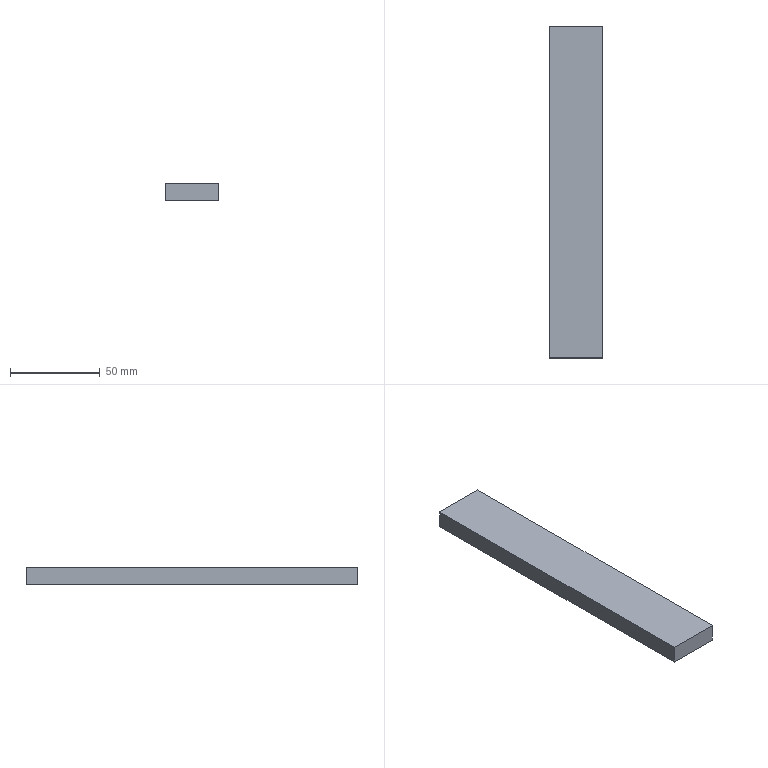Part | NX | features solid 2 | 1 solid | 6 faces | box 30 x 185 x 10 mm | volume 55500 mm3 | plane 6
STEP:
#1=CARTESIAN_POINT('',(665.,-225.,10.));
#2=VERTEX_POINT('',#1);
#3=CARTESIAN_POINT('',(665.,-225.,20.));
#4=VERTEX_POINT('',#3);
#5=CARTESIAN_POINT('',(665.,-225.,-10.));
#6=DIRECTION('',(0.,0.,-1.));
#7=VECTOR('',#6,1000.);
#8=LINE('',#5,#7);
#9=EDGE_CURVE('',#2,#4,#8,.F.);
#10=ORIENTED_EDGE('',*,*,#9,.T.);
#11=CARTESIAN_POINT('',(635.,-225.,20.));
#12=VERTEX_POINT('',#11);
#13=CARTESIAN_POINT('',(675.,-225.,20.));
#14=DIRECTION('',(-1.,0.,0.));
#15=VECTOR('',#14,1000.);
#16=LINE('',#13,#15);
#17=EDGE_CURVE('',#4,#12,#16,.T.);
#18=ORIENTED_EDGE('',*,*,#17,.T.);
#19=CARTESIAN_POINT('',(635.,-225.,10.));
#20=VERTEX_POINT('',#19);
#21=CARTESIAN_POINT('',(635.,-225.,-10.));
#22=DIRECTION('',(0.,0.,1.));
#23=VECTOR('',#22,1000.);
#24=LINE('',#21,#23);
#25=EDGE_CURVE('',#20,#12,#24,.T.);
#26=ORIENTED_EDGE('',*,*,#25,.F.);
#27=CARTESIAN_POINT('',(675.,-225.,10.));
#28=DIRECTION('',(-1.,0.,0.));
#29=VECTOR('',#28,1000.);
#30=LINE('',#27,#29);
#31=EDGE_CURVE('',#2,#20,#30,.T.);
#32=ORIENTED_EDGE('',*,*,#31,.F.);
#33=EDGE_LOOP('',(#10,#18,#26,#32));
#34=FACE_BOUND('',#33,.T.);
#35=CARTESIAN_POINT('',(690.,-225.,-60.));
#36=DIRECTION('',(0.,-1.,0.));
#37=DIRECTION('',(0.,0.,-1.));
#38=AXIS2_PLACEMENT_3D('',#35,#36,#37);
#39=PLANE('',#38);
#40=ADVANCED_FACE('',(#34),#39,.T.);
#41=CARTESIAN_POINT('',(665.,-40.,10.));
#42=VERTEX_POINT('',#41);
#43=CARTESIAN_POINT('',(665.,205.,10.));
#44=DIRECTION('',(0.,1.,0.));
#45=VECTOR('',#44,1000.);
#46=LINE('',#43,#45);
#47=EDGE_CURVE('',#42,#2,#46,.F.);
#48=ORIENTED_EDGE('',*,*,#47,.T.);
#49=ORIENTED_EDGE('',*,*,#31,.T.);
#50=CARTESIAN_POINT('',(635.,-40.,10.));
#51=VERTEX_POINT('',#50);
#52=CARTESIAN_POINT('',(635.,205.,10.));
#53=DIRECTION('',(0.,-1.,0.));
#54=VECTOR('',#53,1000.);
#55=LINE('',#52,#54);
#56=EDGE_CURVE('',#20,#51,#55,.F.);
#57=ORIENTED_EDGE('',*,*,#56,.T.);
#58=CARTESIAN_POINT('',(665.,-40.,10.));
#59=DIRECTION('',(-1.,0.,0.));
#60=VECTOR('',#59,1000.);
#61=LINE('',#58,#60);
#62=EDGE_CURVE('',#42,#51,#61,.T.);
#63=ORIENTED_EDGE('',*,*,#62,.F.);
#64=EDGE_LOOP('',(#48,#49,#57,#63));
#65=FACE_BOUND('',#64,.T.);
#66=CARTESIAN_POINT('',(675.,205.,10.));
#67=DIRECTION('',(0.,0.,-1.));
#68=DIRECTION('',(-1.,0.,0.));
#69=AXIS2_PLACEMENT_3D('',#66,#67,#68);
#70=PLANE('',#69);
#71=ADVANCED_FACE('',(#65),#70,.T.);
#72=CARTESIAN_POINT('',(635.,-40.,20.));
#73=VERTEX_POINT('',#72);
#74=CARTESIAN_POINT('',(635.,-40.,-10.));
#75=DIRECTION('',(0.,0.,-1.));
#76=VECTOR('',#75,1000.);
#77=LINE('',#74,#76);
#78=EDGE_CURVE('',#51,#73,#77,.F.);
#79=ORIENTED_EDGE('',*,*,#78,.F.);
#80=ORIENTED_EDGE('',*,*,#56,.F.);
#81=ORIENTED_EDGE('',*,*,#25,.T.);
#82=CARTESIAN_POINT('',(635.,205.,20.));
#83=DIRECTION('',(0.,-1.,0.));
#84=VECTOR('',#83,1000.);
#85=LINE('',#82,#84);
#86=EDGE_CURVE('',#12,#73,#85,.F.);
#87=ORIENTED_EDGE('',*,*,#86,.T.);
#88=EDGE_LOOP('',(#79,#80,#81,#87));
#89=FACE_BOUND('',#88,.T.);
#90=CARTESIAN_POINT('',(635.,205.,-10.));
#91=DIRECTION('',(1.,0.,0.));
#92=DIRECTION('',(0.,0.,-1.));
#93=AXIS2_PLACEMENT_3D('',#90,#91,#92);
#94=PLANE('',#93);
#95=ADVANCED_FACE('',(#89),#94,.F.);
#96=CARTESIAN_POINT('',(665.,-40.,20.));
#97=VERTEX_POINT('',#96);
#98=CARTESIAN_POINT('',(665.,205.,20.));
#99=DIRECTION('',(0.,-1.,0.));
#100=VECTOR('',#99,1000.);
#101=LINE('',#98,#100);
#102=EDGE_CURVE('',#4,#97,#101,.F.);
#103=ORIENTED_EDGE('',*,*,#102,.T.);
#104=CARTESIAN_POINT('',(675.,-40.,20.));
#105=DIRECTION('',(-1.,0.,0.));
#106=VECTOR('',#105,1000.);
#107=LINE('',#104,#106);
#108=EDGE_CURVE('',#97,#73,#107,.T.);
#109=ORIENTED_EDGE('',*,*,#108,.T.);
#110=ORIENTED_EDGE('',*,*,#86,.F.);
#111=ORIENTED_EDGE('',*,*,#17,.F.);
#112=EDGE_LOOP('',(#103,#109,#110,#111));
#113=FACE_BOUND('',#112,.T.);
#114=CARTESIAN_POINT('',(675.,205.,20.));
#115=DIRECTION('',(0.,0.,-1.));
#116=DIRECTION('',(-1.,0.,0.));
#117=AXIS2_PLACEMENT_3D('',#114,#115,#116);
#118=PLANE('',#117);
#119=ADVANCED_FACE('',(#113),#118,.F.);
#120=ORIENTED_EDGE('',*,*,#47,.F.);
#121=CARTESIAN_POINT('',(665.,-40.,-10.));
#122=DIRECTION('',(0.,0.,-1.));
#123=VECTOR('',#122,1000.);
#124=LINE('',#121,#123);
#125=EDGE_CURVE('',#42,#97,#124,.F.);
#126=ORIENTED_EDGE('',*,*,#125,.T.);
#127=ORIENTED_EDGE('',*,*,#102,.F.);
#128=ORIENTED_EDGE('',*,*,#9,.F.);
#129=EDGE_LOOP('',(#120,#126,#127,#128));
#130=FACE_BOUND('',#129,.T.);
#131=CARTESIAN_POINT('',(665.,205.,-10.));
#132=DIRECTION('',(1.,0.,0.));
#133=DIRECTION('',(0.,0.,-1.));
#134=AXIS2_PLACEMENT_3D('',#131,#132,#133);
#135=PLANE('',#134);
#136=ADVANCED_FACE('',(#130),#135,.T.);
#137=ORIENTED_EDGE('',*,*,#78,.T.);
#138=ORIENTED_EDGE('',*,*,#108,.F.);
#139=ORIENTED_EDGE('',*,*,#125,.F.);
#140=ORIENTED_EDGE('',*,*,#62,.T.);
#141=EDGE_LOOP('',(#137,#138,#139,#140));
#142=FACE_BOUND('',#141,.T.);
#143=CARTESIAN_POINT('',(685.,-40.,-10.));
#144=DIRECTION('',(0.,-1.,0.));
#145=DIRECTION('',(0.,0.,-1.));
#146=AXIS2_PLACEMENT_3D('',#143,#144,#145);
#147=PLANE('',#146);
#148=ADVANCED_FACE('',(#142),#147,.F.);
#149=CLOSED_SHELL('',(#40,#71,#95,#119,#136,#148));
#150=MANIFOLD_SOLID_BREP('',#149);
#151=(LENGTH_UNIT()NAMED_UNIT(*)SI_UNIT(.MILLI.,.METRE.));
#152=UNCERTAINTY_MEASURE_WITH_UNIT(LENGTH_MEASURE(0.00001),#151,'','');
#153=(NAMED_UNIT(*)PLANE_ANGLE_UNIT()SI_UNIT($,.RADIAN.));
#154=(NAMED_UNIT(*)SI_UNIT($,.STERADIAN.)SOLID_ANGLE_UNIT());
#155=(GEOMETRIC_REPRESENTATION_CONTEXT(3)GLOBAL_UNCERTAINTY_ASSIGNED_CONTEXT((#152))GLOBAL_UNIT_ASSIGNED_CONTEXT((#151,#153,#154))REPRESENTATION_CONTEXT('',''));
#156=ADVANCED_BREP_SHAPE_REPRESENTATION('',(#150),#155);